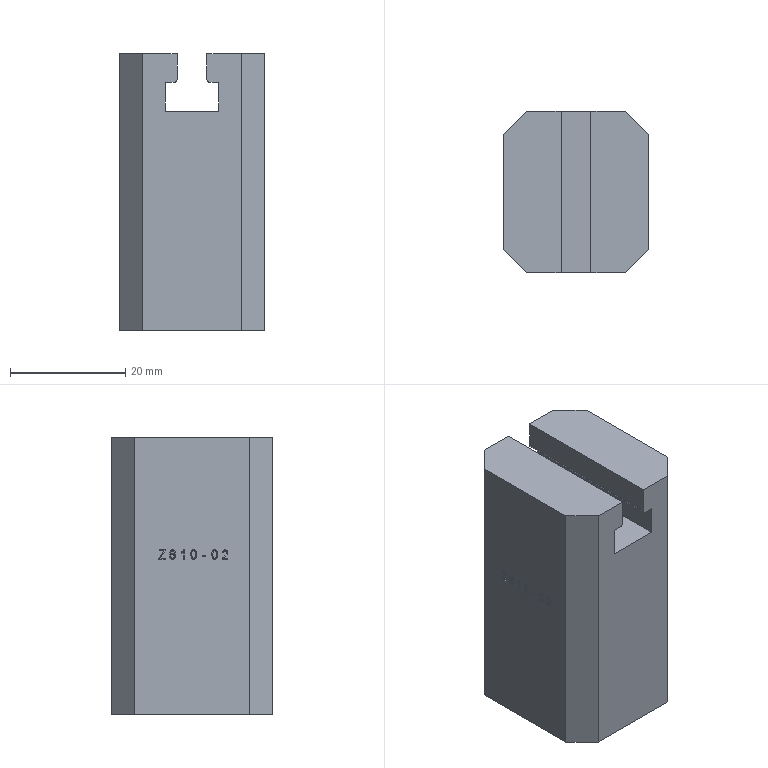Part | Creo | 1 solid | 152 faces | box 25 x 28 x 48 mm | volume 28239 mm3 | other 93 | plane 49 | cylinder 8 | cone 2 | commonest cylinder face diameters 1 x2 8.499 x2 8.5 x2 1.421 x1 22.406 x1